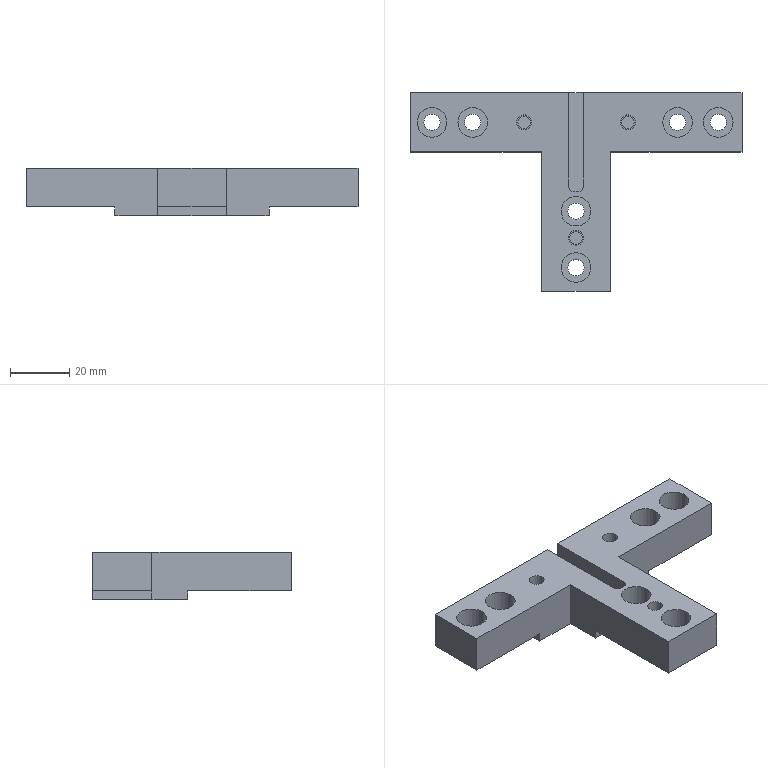Part | SolidWorks | features ICE 7, Extrusion 1 | 1 solid | 70 faces | box 112 x 67 x 16 mm | volume 40788 mm3 | cylinder 38 | plane 32 | commonest cylinder face diameters 5.5 x12 10 x12 4.2 x6 5 x6 4 x2